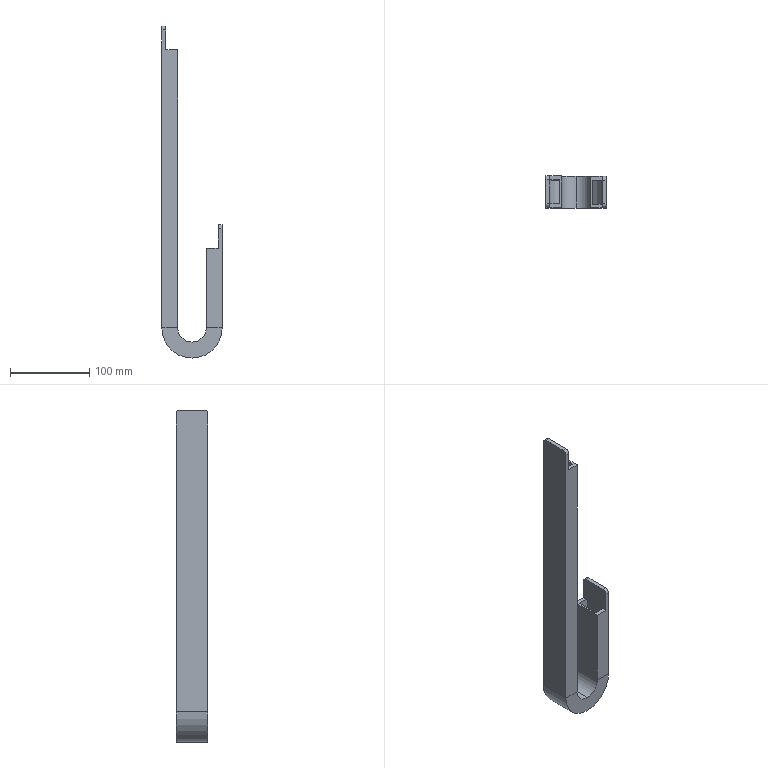Part | SolidWorks | features Fillet 2, ICE 2, Sweep 1, SweepCut 1 | 1 solid | 38 faces | box 76 x 40 x 418 mm | volume 200180 mm3 | plane 28 | cylinder 10 | commonest cylinder face diameters 10 x4 36 x2 76 x2 41 x1 71 x1
STEP:
#1=CARTESIAN_POINT('',(28.,20.,-368.));
#2=VERTEX_POINT('',#1);
#3=CARTESIAN_POINT('',(46.,20.,-350.));
#4=VERTEX_POINT('',#3);
#5=CARTESIAN_POINT('',(28.,20.,-350.));
#6=DIRECTION('',(0.,-1.,0.));
#7=DIRECTION('',(-1.,0.,0.));
#8=AXIS2_PLACEMENT_3D('',#5,#6,#7);
#9=CIRCLE('',#8,18.);
#10=EDGE_CURVE('',#2,#4,#9,.T.);
#11=ORIENTED_EDGE('',*,*,#10,.F.);
#12=CARTESIAN_POINT('',(28.,-20.,-368.));
#13=VERTEX_POINT('',#12);
#14=CARTESIAN_POINT('',(28.,0.,-368.));
#15=DIRECTION('',(0.,-1.,0.));
#16=VECTOR('',#15,1000.);
#17=LINE('',#14,#16);
#18=EDGE_CURVE('',#2,#13,#17,.T.);
#19=ORIENTED_EDGE('',*,*,#18,.T.);
#20=CARTESIAN_POINT('',(46.,-20.,-350.));
#21=VERTEX_POINT('',#20);
#22=CARTESIAN_POINT('',(28.,-20.,-350.));
#23=DIRECTION('',(0.,-1.,0.));
#24=DIRECTION('',(-1.,0.,0.));
#25=AXIS2_PLACEMENT_3D('',#22,#23,#24);
#26=CIRCLE('',#25,18.);
#27=EDGE_CURVE('',#13,#21,#26,.T.);
#28=ORIENTED_EDGE('',*,*,#27,.T.);
#29=CARTESIAN_POINT('',(46.,20.,-350.));
#30=DIRECTION('',(0.,1.,0.));
#31=VECTOR('',#30,1000.);
#32=LINE('',#29,#31);
#33=EDGE_CURVE('',#21,#4,#32,.T.);
#34=ORIENTED_EDGE('',*,*,#33,.T.);
#35=EDGE_LOOP('',(#11,#19,#28,#34));
#36=FACE_OUTER_BOUND('',#35,.T.);
#37=CARTESIAN_POINT('',(28.,0.,-350.));
#38=DIRECTION('',(0.,-1.,0.));
#39=DIRECTION('',(0.,0.,-1.));
#40=AXIS2_PLACEMENT_3D('',#37,#38,#39);
#41=CYLINDRICAL_SURFACE('',#40,18.);
#42=ADVANCED_FACE('',(#36),#41,.F.);
#43=CARTESIAN_POINT('',(-10.,20.,-350.));
#44=VERTEX_POINT('',#43);
#45=CARTESIAN_POINT('',(28.,20.,-388.));
#46=VERTEX_POINT('',#45);
#47=CARTESIAN_POINT('',(28.,20.,-350.));
#48=DIRECTION('',(0.,-1.,0.));
#49=DIRECTION('',(-1.,0.,0.));
#50=AXIS2_PLACEMENT_3D('',#47,#48,#49);
#51=CIRCLE('',#50,38.);
#52=EDGE_CURVE('',#44,#46,#51,.T.);
#53=ORIENTED_EDGE('',*,*,#52,.T.);
#54=CARTESIAN_POINT('',(28.,-20.,-388.));
#55=VERTEX_POINT('',#54);
#56=CARTESIAN_POINT('',(28.,0.,-388.));
#57=DIRECTION('',(0.,-1.,0.));
#58=VECTOR('',#57,1000.);
#59=LINE('',#56,#58);
#60=EDGE_CURVE('',#46,#55,#59,.T.);
#61=ORIENTED_EDGE('',*,*,#60,.T.);
#62=CARTESIAN_POINT('',(-10.,-20.,-350.));
#63=VERTEX_POINT('',#62);
#64=CARTESIAN_POINT('',(28.,-20.,-350.));
#65=DIRECTION('',(0.,-1.,0.));
#66=DIRECTION('',(-1.,0.,0.));
#67=AXIS2_PLACEMENT_3D('',#64,#65,#66);
#68=CIRCLE('',#67,38.);
#69=EDGE_CURVE('',#63,#55,#68,.T.);
#70=ORIENTED_EDGE('',*,*,#69,.F.);
#71=CARTESIAN_POINT('',(-10.,20.,-350.));
#72=DIRECTION('',(0.,-1.,0.));
#73=VECTOR('',#72,1000.);
#74=LINE('',#71,#73);
#75=EDGE_CURVE('',#44,#63,#74,.T.);
#76=ORIENTED_EDGE('',*,*,#75,.F.);
#77=EDGE_LOOP('',(#53,#61,#70,#76));
#78=FACE_OUTER_BOUND('',#77,.T.);
#79=CARTESIAN_POINT('',(28.,0.,-350.));
#80=DIRECTION('',(0.,-1.,0.));
#81=DIRECTION('',(0.,0.,-1.));
#82=AXIS2_PLACEMENT_3D('',#79,#80,#81);
#83=CYLINDRICAL_SURFACE('',#82,38.);
#84=ADVANCED_FACE('',(#78),#83,.T.);
#85=CARTESIAN_POINT('',(61.,20.,-250.));
#86=VERTEX_POINT('',#85);
#87=CARTESIAN_POINT('',(61.,15.,-250.));
#88=VERTEX_POINT('',#87);
#89=CARTESIAN_POINT('',(61.,-20.,-250.));
#90=DIRECTION('',(0.,-1.,0.));
#91=VECTOR('',#90,1000.);
#92=LINE('',#89,#91);
#93=EDGE_CURVE('',#86,#88,#92,.T.);
#94=ORIENTED_EDGE('',*,*,#93,.F.);
#95=CARTESIAN_POINT('',(46.,20.,-250.));
#96=VERTEX_POINT('',#95);
#97=CARTESIAN_POINT('',(66.,20.,-250.));
#98=DIRECTION('',(1.,0.,0.));
#99=VECTOR('',#98,1000.);
#100=LINE('',#97,#99);
#101=EDGE_CURVE('',#96,#86,#100,.T.);
#102=ORIENTED_EDGE('',*,*,#101,.F.);
#103=CARTESIAN_POINT('',(46.,-20.,-250.));
#104=VERTEX_POINT('',#103);
#105=CARTESIAN_POINT('',(46.,20.,-250.));
#106=DIRECTION('',(0.,1.,0.));
#107=VECTOR('',#106,1000.);
#108=LINE('',#105,#107);
#109=EDGE_CURVE('',#104,#96,#108,.T.);
#110=ORIENTED_EDGE('',*,*,#109,.F.);
#111=CARTESIAN_POINT('',(61.,-20.,-250.));
#112=VERTEX_POINT('',#111);
#113=CARTESIAN_POINT('',(66.,-20.,-250.));
#114=DIRECTION('',(-1.,0.,0.));
#115=VECTOR('',#114,1000.);
#116=LINE('',#113,#115);
#117=EDGE_CURVE('',#112,#104,#116,.T.);
#118=ORIENTED_EDGE('',*,*,#117,.F.);
#119=CARTESIAN_POINT('',(61.,-15.,-250.));
#120=VERTEX_POINT('',#119);
#121=CARTESIAN_POINT('',(61.,-20.,-250.));
#122=DIRECTION('',(0.,-1.,0.));
#123=VECTOR('',#122,1000.);
#124=LINE('',#121,#123);
#125=EDGE_CURVE('',#120,#112,#124,.T.);
#126=ORIENTED_EDGE('',*,*,#125,.F.);
#127=CARTESIAN_POINT('',(48.5,-15.,-250.));
#128=VERTEX_POINT('',#127);
#129=CARTESIAN_POINT('',(56.,-15.,-250.));
#130=DIRECTION('',(-1.,0.,0.));
#131=VECTOR('',#130,1000.);
#132=LINE('',#129,#131);
#133=EDGE_CURVE('',#120,#128,#132,.T.);
#134=ORIENTED_EDGE('',*,*,#133,.T.);
#135=CARTESIAN_POINT('',(48.5,15.,-250.));
#136=VERTEX_POINT('',#135);
#137=CARTESIAN_POINT('',(48.5,0.,-250.));
#138=DIRECTION('',(0.,1.,0.));
#139=VECTOR('',#138,1000.);
#140=LINE('',#137,#139);
#141=EDGE_CURVE('',#128,#136,#140,.T.);
#142=ORIENTED_EDGE('',*,*,#141,.T.);
#143=CARTESIAN_POINT('',(56.,15.,-250.));
#144=DIRECTION('',(1.,0.,0.));
#145=VECTOR('',#144,1000.);
#146=LINE('',#143,#145);
#147=EDGE_CURVE('',#136,#88,#146,.T.);
#148=ORIENTED_EDGE('',*,*,#147,.T.);
#149=EDGE_LOOP('',(#94,#102,#110,#118,#126,#134,#142,#148));
#150=FACE_OUTER_BOUND('',#149,.T.);
#151=CARTESIAN_POINT('',(56.,0.,-250.));
#152=DIRECTION('',(0.,0.,-1.));
#153=DIRECTION('',(-1.,0.,0.));
#154=AXIS2_PLACEMENT_3D('',#151,#152,#153);
#155=PLANE('',#154);
#156=ADVANCED_FACE('',(#150),#155,.F.);
#157=CARTESIAN_POINT('',(61.,20.,-225.));
#158=VERTEX_POINT('',#157);
#159=CARTESIAN_POINT('',(61.,20.,-220.));
#160=DIRECTION('',(0.,0.,-1.));
#161=VECTOR('',#160,1000.);
#162=LINE('',#159,#161);
#163=EDGE_CURVE('',#158,#86,#162,.T.);
#164=ORIENTED_EDGE('',*,*,#163,.F.);
#165=CARTESIAN_POINT('',(66.,20.,-225.));
#166=VERTEX_POINT('',#165);
#167=CARTESIAN_POINT('',(66.,20.,-225.));
#168=DIRECTION('',(1.,0.,0.));
#169=VECTOR('',#168,1000.);
#170=LINE('',#167,#169);
#171=EDGE_CURVE('',#158,#166,#170,.T.);
#172=ORIENTED_EDGE('',*,*,#171,.T.);
#173=CARTESIAN_POINT('',(66.,20.,-350.));
#174=VERTEX_POINT('',#173);
#175=CARTESIAN_POINT('',(66.,20.,-350.));
#176=DIRECTION('',(0.,0.,1.));
#177=VECTOR('',#176,1000.);
#178=LINE('',#175,#177);
#179=EDGE_CURVE('',#174,#166,#178,.T.);
#180=ORIENTED_EDGE('',*,*,#179,.F.);
#181=CARTESIAN_POINT('',(66.,20.,-350.));
#182=DIRECTION('',(1.,0.,0.));
#183=VECTOR('',#182,1000.);
#184=LINE('',#181,#183);
#185=EDGE_CURVE('',#4,#174,#184,.T.);
#186=ORIENTED_EDGE('',*,*,#185,.F.);
#187=CARTESIAN_POINT('',(46.,20.,-350.));
#188=DIRECTION('',(0.,0.,1.));
#189=VECTOR('',#188,1000.);
#190=LINE('',#187,#189);
#191=EDGE_CURVE('',#4,#96,#190,.T.);
#192=ORIENTED_EDGE('',*,*,#191,.T.);
#193=ORIENTED_EDGE('',*,*,#101,.T.);
#194=EDGE_LOOP('',(#164,#172,#180,#186,#192,#193));
#195=FACE_OUTER_BOUND('',#194,.T.);
#196=CARTESIAN_POINT('',(66.,20.,-350.));
#197=DIRECTION('',(0.,-1.,0.));
#198=DIRECTION('',(1.,0.,0.));
#199=AXIS2_PLACEMENT_3D('',#196,#197,#198);
#200=PLANE('',#199);
#201=ADVANCED_FACE('',(#195),#200,.F.);
#202=ORIENTED_EDGE('',*,*,#191,.F.);
#203=ORIENTED_EDGE('',*,*,#33,.F.);
#204=CARTESIAN_POINT('',(46.,-20.,-350.));
#205=DIRECTION('',(0.,0.,1.));
#206=VECTOR('',#205,1000.);
#207=LINE('',#204,#206);
#208=EDGE_CURVE('',#21,#104,#207,.T.);
#209=ORIENTED_EDGE('',*,*,#208,.T.);
#210=ORIENTED_EDGE('',*,*,#109,.T.);
#211=EDGE_LOOP('',(#202,#203,#209,#210));
#212=FACE_OUTER_BOUND('',#211,.T.);
#213=CARTESIAN_POINT('',(46.,20.,-350.));
#214=DIRECTION('',(1.,0.,0.));
#215=DIRECTION('',(0.,0.,-1.));
#216=AXIS2_PLACEMENT_3D('',#213,#214,#215);
#217=PLANE('',#216);
#218=ADVANCED_FACE('',(#212),#217,.F.);
#219=CARTESIAN_POINT('',(66.,-20.,-350.));
#220=VERTEX_POINT('',#219);
#221=CARTESIAN_POINT('',(66.,-20.,-225.));
#222=VERTEX_POINT('',#221);
#223=CARTESIAN_POINT('',(66.,-20.,-350.));
#224=DIRECTION('',(0.,0.,1.));
#225=VECTOR('',#224,1000.);
#226=LINE('',#223,#225);
#227=EDGE_CURVE('',#220,#222,#226,.T.);
#228=ORIENTED_EDGE('',*,*,#227,.T.);
#229=CARTESIAN_POINT('',(61.,-20.,-225.));
#230=VERTEX_POINT('',#229);
#231=CARTESIAN_POINT('',(61.,-20.,-225.));
#232=DIRECTION('',(-1.,0.,0.));
#233=VECTOR('',#232,1000.);
#234=LINE('',#231,#233);
#235=EDGE_CURVE('',#222,#230,#234,.T.);
#236=ORIENTED_EDGE('',*,*,#235,.T.);
#237=CARTESIAN_POINT('',(61.,-20.,-220.));
#238=DIRECTION('',(0.,0.,-1.));
#239=VECTOR('',#238,1000.);
#240=LINE('',#237,#239);
#241=EDGE_CURVE('',#230,#112,#240,.T.);
#242=ORIENTED_EDGE('',*,*,#241,.T.);
#243=ORIENTED_EDGE('',*,*,#117,.T.);
#244=ORIENTED_EDGE('',*,*,#208,.F.);
#245=CARTESIAN_POINT('',(66.,-20.,-350.));
#246=DIRECTION('',(-1.,0.,0.));
#247=VECTOR('',#246,1000.);
#248=LINE('',#245,#247);
#249=EDGE_CURVE('',#220,#21,#248,.T.);
#250=ORIENTED_EDGE('',*,*,#249,.F.);
#251=EDGE_LOOP('',(#228,#236,#242,#243,#244,#250));
#252=FACE_OUTER_BOUND('',#251,.T.);
#253=CARTESIAN_POINT('',(66.,-20.,-350.));
#254=DIRECTION('',(0.,1.,0.));
#255=DIRECTION('',(0.,0.,1.));
#256=AXIS2_PLACEMENT_3D('',#253,#254,#255);
#257=PLANE('',#256);
#258=ADVANCED_FACE('',(#252),#257,.F.);
#259=ORIENTED_EDGE('',*,*,#179,.T.);
#260=CARTESIAN_POINT('',(66.,15.,-220.));
#261=VERTEX_POINT('',#260);
#262=CARTESIAN_POINT('',(66.,15.,-225.));
#263=DIRECTION('',(1.,0.,0.));
#264=DIRECTION('',(0.,0.,1.));
#265=AXIS2_PLACEMENT_3D('',#262,#263,#264);
#266=CIRCLE('',#265,5.);
#267=EDGE_CURVE('',#166,#261,#266,.T.);
#268=ORIENTED_EDGE('',*,*,#267,.T.);
#269=CARTESIAN_POINT('',(66.,-15.,-220.));
#270=VERTEX_POINT('',#269);
#271=CARTESIAN_POINT('',(66.,-20.,-220.));
#272=DIRECTION('',(0.,1.,0.));
#273=VECTOR('',#272,1000.);
#274=LINE('',#271,#273);
#275=EDGE_CURVE('',#270,#261,#274,.T.);
#276=ORIENTED_EDGE('',*,*,#275,.F.);
#277=CARTESIAN_POINT('',(66.,-15.,-225.));
#278=DIRECTION('',(1.,0.,0.));
#279=DIRECTION('',(0.,0.,1.));
#280=AXIS2_PLACEMENT_3D('',#277,#278,#279);
#281=CIRCLE('',#280,5.);
#282=EDGE_CURVE('',#270,#222,#281,.T.);
#283=ORIENTED_EDGE('',*,*,#282,.T.);
#284=ORIENTED_EDGE('',*,*,#227,.F.);
#285=CARTESIAN_POINT('',(66.,20.,-350.));
#286=DIRECTION('',(0.,-1.,0.));
#287=VECTOR('',#286,1000.);
#288=LINE('',#285,#287);
#289=EDGE_CURVE('',#174,#220,#288,.T.);
#290=ORIENTED_EDGE('',*,*,#289,.F.);
#291=EDGE_LOOP('',(#259,#268,#276,#283,#284,#290));
#292=FACE_OUTER_BOUND('',#291,.T.);
#293=CARTESIAN_POINT('',(66.,20.,-350.));
#294=DIRECTION('',(-1.,0.,0.));
#295=DIRECTION('',(0.,0.,1.));
#296=AXIS2_PLACEMENT_3D('',#293,#294,#295);
#297=PLANE('',#296);
#298=ADVANCED_FACE('',(#292),#297,.F.);
#299=ORIENTED_EDGE('',*,*,#185,.T.);
#300=CARTESIAN_POINT('',(28.,20.,-350.));
#301=DIRECTION('',(0.,-1.,0.));
#302=DIRECTION('',(-1.,0.,0.));
#303=AXIS2_PLACEMENT_3D('',#300,#301,#302);
#304=CIRCLE('',#303,38.);
#305=EDGE_CURVE('',#46,#174,#304,.T.);
#306=ORIENTED_EDGE('',*,*,#305,.F.);
#307=ORIENTED_EDGE('',*,*,#52,.F.);
#308=CARTESIAN_POINT('',(10.,20.,-350.));
#309=VERTEX_POINT('',#308);
#310=CARTESIAN_POINT('',(-10.,20.,-350.));
#311=DIRECTION('',(-1.,0.,0.));
#312=VECTOR('',#311,1000.);
#313=LINE('',#310,#312);
#314=EDGE_CURVE('',#309,#44,#313,.T.);
#315=ORIENTED_EDGE('',*,*,#314,.F.);
#316=CARTESIAN_POINT('',(28.,20.,-350.));
#317=DIRECTION('',(0.,-1.,0.));
#318=DIRECTION('',(-1.,0.,0.));
#319=AXIS2_PLACEMENT_3D('',#316,#317,#318);
#320=CIRCLE('',#319,18.);
#321=EDGE_CURVE('',#309,#2,#320,.T.);
#322=ORIENTED_EDGE('',*,*,#321,.T.);
#323=ORIENTED_EDGE('',*,*,#10,.T.);
#324=EDGE_LOOP('',(#299,#306,#307,#315,#322,#323));
#325=FACE_OUTER_BOUND('',#324,.T.);
#326=CARTESIAN_POINT('',(-10.,20.,-350.));
#327=DIRECTION('',(0.,-1.,0.));
#328=DIRECTION('',(0.,0.,-1.));
#329=AXIS2_PLACEMENT_3D('',#326,#327,#328);
#330=PLANE('',#329);
#331=ADVANCED_FACE('',(#325),#330,.F.);
#332=ORIENTED_EDGE('',*,*,#18,.F.);
#333=ORIENTED_EDGE('',*,*,#321,.F.);
#334=CARTESIAN_POINT('',(10.,-20.,-350.));
#335=VERTEX_POINT('',#334);
#336=CARTESIAN_POINT('',(10.,20.,-350.));
#337=DIRECTION('',(0.,1.,0.));
#338=VECTOR('',#337,1000.);
#339=LINE('',#336,#338);
#340=EDGE_CURVE('',#335,#309,#339,.T.);
#341=ORIENTED_EDGE('',*,*,#340,.F.);
#342=CARTESIAN_POINT('',(28.,-20.,-350.));
#343=DIRECTION('',(0.,-1.,0.));
#344=DIRECTION('',(-1.,0.,0.));
#345=AXIS2_PLACEMENT_3D('',#342,#343,#344);
#346=CIRCLE('',#345,18.);
#347=EDGE_CURVE('',#335,#13,#346,.T.);
#348=ORIENTED_EDGE('',*,*,#347,.T.);
#349=EDGE_LOOP('',(#332,#333,#341,#348));
#350=FACE_OUTER_BOUND('',#349,.T.);
#351=CARTESIAN_POINT('',(28.,0.,-350.));
#352=DIRECTION('',(0.,-1.,0.));
#353=DIRECTION('',(0.,0.,-1.));
#354=AXIS2_PLACEMENT_3D('',#351,#352,#353);
#355=CYLINDRICAL_SURFACE('',#354,18.);
#356=ADVANCED_FACE('',(#350),#355,.F.);
#357=ORIENTED_EDGE('',*,*,#347,.F.);
#358=CARTESIAN_POINT('',(-10.,-20.,-350.));
#359=DIRECTION('',(1.,0.,0.));
#360=VECTOR('',#359,1000.);
#361=LINE('',#358,#360);
#362=EDGE_CURVE('',#63,#335,#361,.T.);
#363=ORIENTED_EDGE('',*,*,#362,.F.);
#364=ORIENTED_EDGE('',*,*,#69,.T.);
#365=CARTESIAN_POINT('',(28.,-20.,-350.));
#366=DIRECTION('',(0.,-1.,0.));
#367=DIRECTION('',(-1.,0.,0.));
#368=AXIS2_PLACEMENT_3D('',#365,#366,#367);
#369=CIRCLE('',#368,38.);
#370=EDGE_CURVE('',#55,#220,#369,.T.);
#371=ORIENTED_EDGE('',*,*,#370,.T.);
#372=ORIENTED_EDGE('',*,*,#249,.T.);
#373=ORIENTED_EDGE('',*,*,#27,.F.);
#374=EDGE_LOOP('',(#357,#363,#364,#371,#372,#373));
#375=FACE_OUTER_BOUND('',#374,.T.);
#376=CARTESIAN_POINT('',(-10.,-20.,-350.));
#377=DIRECTION('',(0.,1.,0.));
#378=DIRECTION('',(0.,0.,1.));
#379=AXIS2_PLACEMENT_3D('',#376,#377,#378);
#380=PLANE('',#379);
#381=ADVANCED_FACE('',(#375),#380,.F.);
#382=ORIENTED_EDGE('',*,*,#60,.F.);
#383=ORIENTED_EDGE('',*,*,#305,.T.);
#384=ORIENTED_EDGE('',*,*,#289,.T.);
#385=ORIENTED_EDGE('',*,*,#370,.F.);
#386=EDGE_LOOP('',(#382,#383,#384,#385));
#387=FACE_OUTER_BOUND('',#386,.T.);
#388=CARTESIAN_POINT('',(28.,0.,-350.));
#389=DIRECTION('',(0.,-1.,0.));
#390=DIRECTION('',(0.,0.,-1.));
#391=AXIS2_PLACEMENT_3D('',#388,#389,#390);
#392=CYLINDRICAL_SURFACE('',#391,38.);
#393=ADVANCED_FACE('',(#387),#392,.T.);
#394=CARTESIAN_POINT('',(-10.,20.,25.));
#395=VERTEX_POINT('',#394);
#396=CARTESIAN_POINT('',(-10.,20.,0.));
#397=DIRECTION('',(0.,0.,-1.));
#398=VECTOR('',#397,1000.);
#399=LINE('',#396,#398);
#400=EDGE_CURVE('',#395,#44,#399,.T.);
#401=ORIENTED_EDGE('',*,*,#400,.F.);
#402=CARTESIAN_POINT('',(-5.,20.,25.));
#403=VERTEX_POINT('',#402);
#404=CARTESIAN_POINT('',(-10.,20.,25.));
#405=DIRECTION('',(1.,0.,0.));
#406=VECTOR('',#405,1000.);
#407=LINE('',#404,#406);
#408=EDGE_CURVE('',#395,#403,#407,.T.);
#409=ORIENTED_EDGE('',*,*,#408,.T.);
#410=CARTESIAN_POINT('',(-5.,20.,0.));
#411=VERTEX_POINT('',#410);
#412=CARTESIAN_POINT('',(-5.,20.,30.));
#413=DIRECTION('',(0.,0.,-1.));
#414=VECTOR('',#413,1000.);
#415=LINE('',#412,#414);
#416=EDGE_CURVE('',#403,#411,#415,.T.);
#417=ORIENTED_EDGE('',*,*,#416,.T.);
#418=CARTESIAN_POINT('',(10.,20.,0.));
#419=VERTEX_POINT('',#418);
#420=CARTESIAN_POINT('',(-10.,20.,0.));
#421=DIRECTION('',(-1.,0.,0.));
#422=VECTOR('',#421,1000.);
#423=LINE('',#420,#422);
#424=EDGE_CURVE('',#419,#411,#423,.T.);
#425=ORIENTED_EDGE('',*,*,#424,.F.);
#426=CARTESIAN_POINT('',(10.,20.,0.));
#427=DIRECTION('',(0.,0.,-1.));
#428=VECTOR('',#427,1000.);
#429=LINE('',#426,#428);
#430=EDGE_CURVE('',#419,#309,#429,.T.);
#431=ORIENTED_EDGE('',*,*,#430,.T.);
#432=ORIENTED_EDGE('',*,*,#314,.T.);
#433=EDGE_LOOP('',(#401,#409,#417,#425,#431,#432));
#434=FACE_OUTER_BOUND('',#433,.T.);
#435=CARTESIAN_POINT('',(-10.,20.,0.));
#436=DIRECTION('',(0.,-1.,0.));
#437=DIRECTION('',(1.,0.,0.));
#438=AXIS2_PLACEMENT_3D('',#435,#436,#437);
#439=PLANE('',#438);
#440=ADVANCED_FACE('',(#434),#439,.F.);
#441=ORIENTED_EDGE('',*,*,#430,.F.);
#442=CARTESIAN_POINT('',(10.,-20.,0.));
#443=VERTEX_POINT('',#442);
#444=CARTESIAN_POINT('',(10.,20.,0.));
#445=DIRECTION('',(0.,1.,0.));
#446=VECTOR('',#445,1000.);
#447=LINE('',#444,#446);
#448=EDGE_CURVE('',#443,#419,#447,.T.);
#449=ORIENTED_EDGE('',*,*,#448,.F.);
#450=CARTESIAN_POINT('',(10.,-20.,0.));
#451=DIRECTION('',(0.,0.,-1.));
#452=VECTOR('',#451,1000.);
#453=LINE('',#450,#452);
#454=EDGE_CURVE('',#443,#335,#453,.T.);
#455=ORIENTED_EDGE('',*,*,#454,.T.);
#456=ORIENTED_EDGE('',*,*,#340,.T.);
#457=EDGE_LOOP('',(#441,#449,#455,#456));
#458=FACE_OUTER_BOUND('',#457,.T.);
#459=CARTESIAN_POINT('',(10.,20.,0.));
#460=DIRECTION('',(-1.,0.,0.));
#461=DIRECTION('',(0.,-1.,0.));
#462=AXIS2_PLACEMENT_3D('',#459,#460,#461);
#463=PLANE('',#462);
#464=ADVANCED_FACE('',(#458),#463,.F.);
#465=CARTESIAN_POINT('',(-5.,-20.,25.));
#466=VERTEX_POINT('',#465);
#467=CARTESIAN_POINT('',(-5.,-20.,0.));
#468=VERTEX_POINT('',#467);
#469=CARTESIAN_POINT('',(-5.,-20.,30.));
#470=DIRECTION('',(0.,0.,-1.));
#471=VECTOR('',#470,1000.);
#472=LINE('',#469,#471);
#473=EDGE_CURVE('',#466,#468,#472,.T.);
#474=ORIENTED_EDGE('',*,*,#473,.F.);
#475=CARTESIAN_POINT('',(-10.,-20.,25.));
#476=VERTEX_POINT('',#475);
#477=CARTESIAN_POINT('',(-10.,-20.,25.));
#478=DIRECTION('',(-1.,0.,0.));
#479=VECTOR('',#478,1000.);
#480=LINE('',#477,#479);
#481=EDGE_CURVE('',#466,#476,#480,.T.);
#482=ORIENTED_EDGE('',*,*,#481,.T.);
#483=CARTESIAN_POINT('',(-10.,-20.,0.));
#484=DIRECTION('',(0.,0.,-1.));
#485=VECTOR('',#484,1000.);
#486=LINE('',#483,#485);
#487=EDGE_CURVE('',#476,#63,#486,.T.);
#488=ORIENTED_EDGE('',*,*,#487,.T.);
#489=ORIENTED_EDGE('',*,*,#362,.T.);
#490=ORIENTED_EDGE('',*,*,#454,.F.);
#491=CARTESIAN_POINT('',(-10.,-20.,0.));
#492=DIRECTION('',(1.,0.,0.));
#493=VECTOR('',#492,1000.);
#494=LINE('',#491,#493);
#495=EDGE_CURVE('',#468,#443,#494,.T.);
#496=ORIENTED_EDGE('',*,*,#495,.F.);
#497=EDGE_LOOP('',(#474,#482,#488,#489,#490,#496));
#498=FACE_OUTER_BOUND('',#497,.T.);
#499=CARTESIAN_POINT('',(-10.,-20.,0.));
#500=DIRECTION('',(0.,1.,0.));
#501=DIRECTION('',(0.,0.,1.));
#502=AXIS2_PLACEMENT_3D('',#499,#500,#501);
#503=PLANE('',#502);
#504=ADVANCED_FACE('',(#498),#503,.F.);
#505=ORIENTED_EDGE('',*,*,#487,.F.);
#506=CARTESIAN_POINT('',(-10.,-15.,30.));
#507=VERTEX_POINT('',#506);
#508=CARTESIAN_POINT('',(-10.,-15.,25.));
#509=DIRECTION('',(-1.,0.,0.));
#510=DIRECTION('',(0.,1.,0.));
#511=AXIS2_PLACEMENT_3D('',#508,#509,#510);
#512=CIRCLE('',#511,5.);
#513=EDGE_CURVE('',#476,#507,#512,.T.);
#514=ORIENTED_EDGE('',*,*,#513,.T.);
#515=CARTESIAN_POINT('',(-10.,15.,30.));
#516=VERTEX_POINT('',#515);
#517=CARTESIAN_POINT('',(-10.,20.,30.));
#518=DIRECTION('',(0.,-1.,0.));
#519=VECTOR('',#518,1000.);
#520=LINE('',#517,#519);
#521=EDGE_CURVE('',#516,#507,#520,.T.);
#522=ORIENTED_EDGE('',*,*,#521,.F.);
#523=CARTESIAN_POINT('',(-10.,15.,25.));
#524=DIRECTION('',(-1.,0.,0.));
#525=DIRECTION('',(0.,1.,0.));
#526=AXIS2_PLACEMENT_3D('',#523,#524,#525);
#527=CIRCLE('',#526,5.);
#528=EDGE_CURVE('',#516,#395,#527,.T.);
#529=ORIENTED_EDGE('',*,*,#528,.T.);
#530=ORIENTED_EDGE('',*,*,#400,.T.);
#531=ORIENTED_EDGE('',*,*,#75,.T.);
#532=EDGE_LOOP('',(#505,#514,#522,#529,#530,#531));
#533=FACE_OUTER_BOUND('',#532,.T.);
#534=CARTESIAN_POINT('',(-10.,20.,0.));
#535=DIRECTION('',(1.,0.,0.));
#536=DIRECTION('',(0.,1.,0.));
#537=AXIS2_PLACEMENT_3D('',#534,#535,#536);
#538=PLANE('',#537);
#539=ADVANCED_FACE('',(#533),#538,.F.);
#540=CARTESIAN_POINT('',(-5.,-15.,0.));
#541=VERTEX_POINT('',#540);
#542=CARTESIAN_POINT('',(-5.,20.,0.));
#543=DIRECTION('',(0.,1.,0.));
#544=VECTOR('',#543,1000.);
#545=LINE('',#542,#544);
#546=EDGE_CURVE('',#468,#541,#545,.T.);
#547=ORIENTED_EDGE('',*,*,#546,.F.);
#548=ORIENTED_EDGE('',*,*,#495,.T.);
#549=ORIENTED_EDGE('',*,*,#448,.T.);
#550=ORIENTED_EDGE('',*,*,#424,.T.);
#551=CARTESIAN_POINT('',(-5.,15.,0.));
#552=VERTEX_POINT('',#551);
#553=CARTESIAN_POINT('',(-5.,20.,0.));
#554=DIRECTION('',(0.,1.,0.));
#555=VECTOR('',#554,1000.);
#556=LINE('',#553,#555);
#557=EDGE_CURVE('',#552,#411,#556,.T.);
#558=ORIENTED_EDGE('',*,*,#557,.F.);
#559=CARTESIAN_POINT('',(7.5,15.,0.));
#560=VERTEX_POINT('',#559);
#561=CARTESIAN_POINT('',(7.5,15.,0.));
#562=DIRECTION('',(1.,0.,0.));
#563=VECTOR('',#562,1000.);
#564=LINE('',#561,#563);
#565=EDGE_CURVE('',#552,#560,#564,.T.);
#566=ORIENTED_EDGE('',*,*,#565,.T.);
#567=CARTESIAN_POINT('',(7.5,-15.,0.));
#568=VERTEX_POINT('',#567);
#569=CARTESIAN_POINT('',(7.5,15.,0.));
#570=DIRECTION('',(0.,-1.,0.));
#571=VECTOR('',#570,1000.);
#572=LINE('',#569,#571);
#573=EDGE_CURVE('',#560,#568,#572,.T.);
#574=ORIENTED_EDGE('',*,*,#573,.T.);
#575=CARTESIAN_POINT('',(7.5,-15.,0.));
#576=DIRECTION('',(-1.,0.,0.));
#577=VECTOR('',#576,1000.);
#578=LINE('',#575,#577);
#579=EDGE_CURVE('',#568,#541,#578,.T.);
#580=ORIENTED_EDGE('',*,*,#579,.T.);
#581=EDGE_LOOP('',(#547,#548,#549,#550,#558,#566,#574,#580));
#582=FACE_OUTER_BOUND('',#581,.T.);
#583=CARTESIAN_POINT('',(0.,0.,0.));
#584=DIRECTION('',(0.,0.,1.));
#585=DIRECTION('',(1.,0.,0.));
#586=AXIS2_PLACEMENT_3D('',#583,#584,#585);
#587=PLANE('',#586);
#588=ADVANCED_FACE('',(#582),#587,.T.);
#589=CARTESIAN_POINT('',(63.5,15.,-250.));
#590=VERTEX_POINT('',#589);
#591=CARTESIAN_POINT('',(63.5,15.,-350.));
#592=VERTEX_POINT('',#591);
#593=CARTESIAN_POINT('',(63.5,15.,-243.981));
#594=DIRECTION('',(0.,0.,-1.));
#595=VECTOR('',#594,1000.);
#596=LINE('',#593,#595);
#597=EDGE_CURVE('',#590,#592,#596,.T.);
#598=ORIENTED_EDGE('',*,*,#597,.T.);
#599=CARTESIAN_POINT('',(63.5,-15.,-350.));
#600=VERTEX_POINT('',#599);
#601=CARTESIAN_POINT('',(63.5,15.,-350.));
#602=DIRECTION('',(0.,-1.,0.));
#603=VECTOR('',#602,1000.);
#604=LINE('',#601,#603);
#605=EDGE_CURVE('',#592,#600,#604,.T.);
#606=ORIENTED_EDGE('',*,*,#605,.T.);
#607=CARTESIAN_POINT('',(63.5,-15.,-250.));
#608=VERTEX_POINT('',#607);
#609=CARTESIAN_POINT('',(63.5,-15.,-243.981));
#610=DIRECTION('',(0.,0.,-1.));
#611=VECTOR('',#610,1000.);
#612=LINE('',#609,#611);
#613=EDGE_CURVE('',#608,#600,#612,.T.);
#614=ORIENTED_EDGE('',*,*,#613,.F.);
#615=CARTESIAN_POINT('',(63.5,0.,-250.));
#616=DIRECTION('',(0.,-1.,0.));
#617=VECTOR('',#616,1000.);
#618=LINE('',#615,#617);
#619=EDGE_CURVE('',#590,#608,#618,.T.);
#620=ORIENTED_EDGE('',*,*,#619,.F.);
#621=EDGE_LOOP('',(#598,#606,#614,#620));
#622=FACE_OUTER_BOUND('',#621,.T.);
#623=CARTESIAN_POINT('',(63.5,15.,-243.981));
#624=DIRECTION('',(1.,0.,0.));
#625=DIRECTION('',(0.,1.,0.));
#626=AXIS2_PLACEMENT_3D('',#623,#624,#625);
#627=PLANE('',#626);
#628=ADVANCED_FACE('',(#622),#627,.F.);
#629=ORIENTED_EDGE('',*,*,#613,.T.);
#630=CARTESIAN_POINT('',(48.5,-15.,-350.));
#631=VERTEX_POINT('',#630);
#632=CARTESIAN_POINT('',(48.5,-15.,-350.));
#633=DIRECTION('',(-1.,0.,0.));
#634=VECTOR('',#633,1000.);
#635=LINE('',#632,#634);
#636=EDGE_CURVE('',#600,#631,#635,.T.);
#637=ORIENTED_EDGE('',*,*,#636,.T.);
#638=CARTESIAN_POINT('',(48.5,-15.,-243.981));
#639=DIRECTION('',(0.,0.,-1.));
#640=VECTOR('',#639,1000.);
#641=LINE('',#638,#640);
#642=EDGE_CURVE('',#128,#631,#641,.T.);
#643=ORIENTED_EDGE('',*,*,#642,.F.);
#644=ORIENTED_EDGE('',*,*,#133,.F.);
#645=CARTESIAN_POINT('',(56.,-15.,-250.));
#646=DIRECTION('',(-1.,0.,0.));
#647=VECTOR('',#646,1000.);
#648=LINE('',#645,#647);
#649=EDGE_CURVE('',#608,#120,#648,.T.);
#650=ORIENTED_EDGE('',*,*,#649,.F.);
#651=EDGE_LOOP('',(#629,#637,#643,#644,#650));
#652=FACE_OUTER_BOUND('',#651,.T.);
#653=CARTESIAN_POINT('',(48.5,-15.,-243.981));
#654=DIRECTION('',(0.,-1.,0.));
#655=DIRECTION('',(0.,0.,-1.));
#656=AXIS2_PLACEMENT_3D('',#653,#654,#655);
#657=PLANE('',#656);
#658=ADVANCED_FACE('',(#652),#657,.F.);
#659=ORIENTED_EDGE('',*,*,#642,.T.);
#660=CARTESIAN_POINT('',(48.5,15.,-350.));
#661=VERTEX_POINT('',#660);
#662=CARTESIAN_POINT('',(48.5,15.,-350.));
#663=DIRECTION('',(0.,1.,0.));
#664=VECTOR('',#663,1000.);
#665=LINE('',#662,#664);
#666=EDGE_CURVE('',#631,#661,#665,.T.);
#667=ORIENTED_EDGE('',*,*,#666,.T.);
#668=CARTESIAN_POINT('',(48.5,15.,-243.981));
#669=DIRECTION('',(0.,0.,-1.));
#670=VECTOR('',#669,1000.);
#671=LINE('',#668,#670);
#672=EDGE_CURVE('',#136,#661,#671,.T.);
#673=ORIENTED_EDGE('',*,*,#672,.F.);
#674=ORIENTED_EDGE('',*,*,#141,.F.);
#675=EDGE_LOOP('',(#659,#667,#673,#674));
#676=FACE_OUTER_BOUND('',#675,.T.);
#677=CARTESIAN_POINT('',(48.5,15.,-243.981));
#678=DIRECTION('',(-1.,0.,0.));
#679=DIRECTION('',(0.,-1.,0.));
#680=AXIS2_PLACEMENT_3D('',#677,#678,#679);
#681=PLANE('',#680);
#682=ADVANCED_FACE('',(#676),#681,.F.);
#683=ORIENTED_EDGE('',*,*,#672,.T.);
#684=CARTESIAN_POINT('',(48.5,15.,-350.));
#685=DIRECTION('',(1.,0.,0.));
#686=VECTOR('',#685,1000.);
#687=LINE('',#684,#686);
#688=EDGE_CURVE('',#661,#592,#687,.T.);
#689=ORIENTED_EDGE('',*,*,#688,.T.);
#690=ORIENTED_EDGE('',*,*,#597,.F.);
#691=CARTESIAN_POINT('',(56.,15.,-250.));
#692=DIRECTION('',(1.,0.,0.));
#693=VECTOR('',#692,1000.);
#694=LINE('',#691,#693);
#695=EDGE_CURVE('',#88,#590,#694,.T.);
#696=ORIENTED_EDGE('',*,*,#695,.F.);
#697=ORIENTED_EDGE('',*,*,#147,.F.);
#698=EDGE_LOOP('',(#683,#689,#690,#696,#697));
#699=FACE_OUTER_BOUND('',#698,.T.);
#700=CARTESIAN_POINT('',(48.5,15.,-243.981));
#701=DIRECTION('',(0.,1.,0.));
#702=DIRECTION('',(0.,0.,1.));
#703=AXIS2_PLACEMENT_3D('',#700,#701,#702);
#704=PLANE('',#703);
#705=ADVANCED_FACE('',(#699),#704,.F.);
#706=CARTESIAN_POINT('',(-7.5,-15.,-350.));
#707=VERTEX_POINT('',#706);
#708=CARTESIAN_POINT('',(-7.5,-15.,0.));
#709=VERTEX_POINT('',#708);
#710=CARTESIAN_POINT('',(-7.5,-15.,-350.));
#711=DIRECTION('',(0.,0.,1.));
#712=VECTOR('',#711,1000.);
#713=LINE('',#710,#712);
#714=EDGE_CURVE('',#707,#709,#713,.T.);
#715=ORIENTED_EDGE('',*,*,#714,.F.);
#716=CARTESIAN_POINT('',(-7.5,15.,-350.));
#717=VERTEX_POINT('',#716);
#718=CARTESIAN_POINT('',(-7.5,15.,-350.));
#719=DIRECTION('',(0.,-1.,0.));
#720=VECTOR('',#719,1000.);
#721=LINE('',#718,#720);
#722=EDGE_CURVE('',#717,#707,#721,.T.);
#723=ORIENTED_EDGE('',*,*,#722,.F.);
#724=CARTESIAN_POINT('',(-7.5,15.,0.));
#725=VERTEX_POINT('',#724);
#726=CARTESIAN_POINT('',(-7.5,15.,-350.));
#727=DIRECTION('',(0.,0.,1.));
#728=VECTOR('',#727,1000.);
#729=LINE('',#726,#728);
#730=EDGE_CURVE('',#717,#725,#729,.T.);
#731=ORIENTED_EDGE('',*,*,#730,.T.);
#732=CARTESIAN_POINT('',(-7.5,15.,0.));
#733=DIRECTION('',(0.,1.,0.));
#734=VECTOR('',#733,1000.);
#735=LINE('',#732,#734);
#736=EDGE_CURVE('',#709,#725,#735,.T.);
#737=ORIENTED_EDGE('',*,*,#736,.F.);
#738=EDGE_LOOP('',(#715,#723,#731,#737));
#739=FACE_OUTER_BOUND('',#738,.T.);
#740=CARTESIAN_POINT('',(-7.5,15.,-350.));
#741=DIRECTION('',(-1.,0.,0.));
#742=DIRECTION('',(0.,-1.,0.));
#743=AXIS2_PLACEMENT_3D('',#740,#741,#742);
#744=PLANE('',#743);
#745=ADVANCED_FACE('',(#739),#744,.F.);
#746=CARTESIAN_POINT('',(7.5,-15.,-350.));
#747=VERTEX_POINT('',#746);
#748=CARTESIAN_POINT('',(7.5,-15.,-350.));
#749=DIRECTION('',(0.,0.,1.));
#750=VECTOR('',#749,1000.);
#751=LINE('',#748,#750);
#752=EDGE_CURVE('',#747,#568,#751,.T.);
#753=ORIENTED_EDGE('',*,*,#752,.F.);
#754=CARTESIAN_POINT('',(7.5,-15.,-350.));
#755=DIRECTION('',(1.,0.,0.));
#756=VECTOR('',#755,1000.);
#757=LINE('',#754,#756);
#758=EDGE_CURVE('',#707,#747,#757,.T.);
#759=ORIENTED_EDGE('',*,*,#758,.F.);
#760=ORIENTED_EDGE('',*,*,#714,.T.);
#761=CARTESIAN_POINT('',(7.5,-15.,0.));
#762=DIRECTION('',(-1.,0.,0.));
#763=VECTOR('',#762,1000.);
#764=LINE('',#761,#763);
#765=EDGE_CURVE('',#541,#709,#764,.T.);
#766=ORIENTED_EDGE('',*,*,#765,.F.);
#767=ORIENTED_EDGE('',*,*,#579,.F.);
#768=EDGE_LOOP('',(#753,#759,#760,#766,#767));
#769=FACE_OUTER_BOUND('',#768,.T.);
#770=CARTESIAN_POINT('',(7.5,-15.,-350.));
#771=DIRECTION('',(0.,-1.,0.));
#772=DIRECTION('',(0.,0.,-1.));
#773=AXIS2_PLACEMENT_3D('',#770,#771,#772);
#774=PLANE('',#773);
#775=ADVANCED_FACE('',(#769),#774,.F.);
#776=CARTESIAN_POINT('',(7.5,15.,-350.));
#777=VERTEX_POINT('',#776);
#778=CARTESIAN_POINT('',(7.5,15.,-350.));
#779=DIRECTION('',(0.,0.,1.));
#780=VECTOR('',#779,1000.);
#781=LINE('',#778,#780);
#782=EDGE_CURVE('',#777,#560,#781,.T.);
#783=ORIENTED_EDGE('',*,*,#782,.F.);
#784=CARTESIAN_POINT('',(7.5,15.,-350.));
#785=DIRECTION('',(0.,1.,0.));
#786=VECTOR('',#785,1000.);
#787=LINE('',#784,#786);
#788=EDGE_CURVE('',#747,#777,#787,.T.);
#789=ORIENTED_EDGE('',*,*,#788,.F.);
#790=ORIENTED_EDGE('',*,*,#752,.T.);
#791=ORIENTED_EDGE('',*,*,#573,.F.);
#792=EDGE_LOOP('',(#783,#789,#790,#791));
#793=FACE_OUTER_BOUND('',#792,.T.);
#794=CARTESIAN_POINT('',(7.5,15.,-350.));
#795=DIRECTION('',(1.,0.,0.));
#796=DIRECTION('',(0.,1.,0.));
#797=AXIS2_PLACEMENT_3D('',#794,#795,#796);
#798=PLANE('',#797);
#799=ADVANCED_FACE('',(#793),#798,.F.);
#800=ORIENTED_EDGE('',*,*,#730,.F.);
#801=CARTESIAN_POINT('',(7.5,15.,-350.));
#802=DIRECTION('',(-1.,0.,0.));
#803=VECTOR('',#802,1000.);
#804=LINE('',#801,#803);
#805=EDGE_CURVE('',#777,#717,#804,.T.);
#806=ORIENTED_EDGE('',*,*,#805,.F.);
#807=ORIENTED_EDGE('',*,*,#782,.T.);
#808=ORIENTED_EDGE('',*,*,#565,.F.);
#809=CARTESIAN_POINT('',(7.5,15.,0.));
#810=DIRECTION('',(1.,0.,0.));
#811=VECTOR('',#810,1000.);
#812=LINE('',#809,#811);
#813=EDGE_CURVE('',#725,#552,#812,.T.);
#814=ORIENTED_EDGE('',*,*,#813,.F.);
#815=EDGE_LOOP('',(#800,#806,#807,#808,#814));
#816=FACE_OUTER_BOUND('',#815,.T.);
#817=CARTESIAN_POINT('',(7.5,15.,-350.));
#818=DIRECTION('',(0.,1.,0.));
#819=DIRECTION('',(0.,0.,1.));
#820=AXIS2_PLACEMENT_3D('',#817,#818,#819);
#821=PLANE('',#820);
#822=ADVANCED_FACE('',(#816),#821,.F.);
#823=ORIENTED_EDGE('',*,*,#805,.T.);
#824=CARTESIAN_POINT('',(28.,15.,-350.));
#825=DIRECTION('',(0.,1.,0.));
#826=DIRECTION('',(1.,0.,0.));
#827=AXIS2_PLACEMENT_3D('',#824,#825,#826);
#828=CIRCLE('',#827,35.5);
#829=EDGE_CURVE('',#592,#717,#828,.T.);
#830=ORIENTED_EDGE('',*,*,#829,.F.);
#831=ORIENTED_EDGE('',*,*,#688,.F.);
#832=CARTESIAN_POINT('',(28.,15.,-350.));
#833=DIRECTION('',(0.,1.,0.));
#834=DIRECTION('',(1.,0.,0.));
#835=AXIS2_PLACEMENT_3D('',#832,#833,#834);
#836=CIRCLE('',#835,20.5);
#837=EDGE_CURVE('',#661,#777,#836,.T.);
#838=ORIENTED_EDGE('',*,*,#837,.T.);
#839=EDGE_LOOP('',(#823,#830,#831,#838));
#840=FACE_OUTER_BOUND('',#839,.T.);
#841=CARTESIAN_POINT('',(48.5,15.,-350.));
#842=DIRECTION('',(0.,1.,0.));
#843=DIRECTION('',(0.,0.,1.));
#844=AXIS2_PLACEMENT_3D('',#841,#842,#843);
#845=PLANE('',#844);
#846=ADVANCED_FACE('',(#840),#845,.F.);
#847=ORIENTED_EDGE('',*,*,#837,.F.);
#848=ORIENTED_EDGE('',*,*,#666,.F.);
#849=CARTESIAN_POINT('',(28.,-15.,-350.));
#850=DIRECTION('',(0.,1.,0.));
#851=DIRECTION('',(1.,0.,0.));
#852=AXIS2_PLACEMENT_3D('',#849,#850,#851);
#853=CIRCLE('',#852,20.5);
#854=EDGE_CURVE('',#631,#747,#853,.T.);
#855=ORIENTED_EDGE('',*,*,#854,.T.);
#856=ORIENTED_EDGE('',*,*,#788,.T.);
#857=EDGE_LOOP('',(#847,#848,#855,#856));
#858=FACE_OUTER_BOUND('',#857,.T.);
#859=CARTESIAN_POINT('',(28.,0.,-350.));
#860=DIRECTION('',(0.,1.,0.));
#861=DIRECTION('',(0.,0.,1.));
#862=AXIS2_PLACEMENT_3D('',#859,#860,#861);
#863=CYLINDRICAL_SURFACE('',#862,20.5);
#864=ADVANCED_FACE('',(#858),#863,.T.);
#865=ORIENTED_EDGE('',*,*,#854,.F.);
#866=ORIENTED_EDGE('',*,*,#636,.F.);
#867=CARTESIAN_POINT('',(28.,-15.,-350.));
#868=DIRECTION('',(0.,1.,0.));
#869=DIRECTION('',(1.,0.,0.));
#870=AXIS2_PLACEMENT_3D('',#867,#868,#869);
#871=CIRCLE('',#870,35.5);
#872=EDGE_CURVE('',#600,#707,#871,.T.);
#873=ORIENTED_EDGE('',*,*,#872,.T.);
#874=ORIENTED_EDGE('',*,*,#758,.T.);
#875=EDGE_LOOP('',(#865,#866,#873,#874));
#876=FACE_OUTER_BOUND('',#875,.T.);
#877=CARTESIAN_POINT('',(48.5,-15.,-350.));
#878=DIRECTION('',(0.,-1.,0.));
#879=DIRECTION('',(0.,0.,-1.));
#880=AXIS2_PLACEMENT_3D('',#877,#878,#879);
#881=PLANE('',#880);
#882=ADVANCED_FACE('',(#876),#881,.F.);
#883=ORIENTED_EDGE('',*,*,#872,.F.);
#884=ORIENTED_EDGE('',*,*,#605,.F.);
#885=ORIENTED_EDGE('',*,*,#829,.T.);
#886=ORIENTED_EDGE('',*,*,#722,.T.);
#887=EDGE_LOOP('',(#883,#884,#885,#886));
#888=FACE_OUTER_BOUND('',#887,.T.);
#889=CARTESIAN_POINT('',(28.,0.,-350.));
#890=DIRECTION('',(0.,1.,0.));
#891=DIRECTION('',(0.,0.,1.));
#892=AXIS2_PLACEMENT_3D('',#889,#890,#891);
#893=CYLINDRICAL_SURFACE('',#892,35.5);
#894=ADVANCED_FACE('',(#888),#893,.F.);
#895=CARTESIAN_POINT('',(-5.,-15.,30.));
#896=VERTEX_POINT('',#895);
#897=CARTESIAN_POINT('',(-5.,15.,30.));
#898=VERTEX_POINT('',#897);
#899=CARTESIAN_POINT('',(-5.,20.,30.));
#900=DIRECTION('',(0.,1.,0.));
#901=VECTOR('',#900,1000.);
#902=LINE('',#899,#901);
#903=EDGE_CURVE('',#896,#898,#902,.T.);
#904=ORIENTED_EDGE('',*,*,#903,.F.);
#905=CARTESIAN_POINT('',(-5.,-15.,25.));
#906=DIRECTION('',(1.,0.,0.));
#907=DIRECTION('',(0.,-1.,0.));
#908=AXIS2_PLACEMENT_3D('',#905,#906,#907);
#909=CIRCLE('',#908,5.);
#910=EDGE_CURVE('',#896,#466,#909,.T.);
#911=ORIENTED_EDGE('',*,*,#910,.T.);
#912=ORIENTED_EDGE('',*,*,#473,.T.);
#913=ORIENTED_EDGE('',*,*,#546,.T.);
#914=CARTESIAN_POINT('',(-5.,20.,0.));
#915=DIRECTION('',(0.,1.,0.));
#916=VECTOR('',#915,1000.);
#917=LINE('',#914,#916);
#918=EDGE_CURVE('',#541,#552,#917,.T.);
#919=ORIENTED_EDGE('',*,*,#918,.T.);
#920=ORIENTED_EDGE('',*,*,#557,.T.);
#921=ORIENTED_EDGE('',*,*,#416,.F.);
#922=CARTESIAN_POINT('',(-5.,15.,25.));
#923=DIRECTION('',(1.,0.,0.));
#924=DIRECTION('',(0.,-1.,0.));
#925=AXIS2_PLACEMENT_3D('',#922,#923,#924);
#926=CIRCLE('',#925,5.);
#927=EDGE_CURVE('',#403,#898,#926,.T.);
#928=ORIENTED_EDGE('',*,*,#927,.T.);
#929=EDGE_LOOP('',(#904,#911,#912,#913,#919,#920,#921,#928));
#930=FACE_OUTER_BOUND('',#929,.T.);
#931=CARTESIAN_POINT('',(-5.,20.,30.));
#932=DIRECTION('',(-1.,0.,0.));
#933=DIRECTION('',(0.,-1.,0.));
#934=AXIS2_PLACEMENT_3D('',#931,#932,#933);
#935=PLANE('',#934);
#936=ADVANCED_FACE('',(#930),#935,.F.);
#937=ORIENTED_EDGE('',*,*,#521,.T.);
#938=CARTESIAN_POINT('',(0.,-15.,30.));
#939=DIRECTION('',(1.,0.,0.));
#940=VECTOR('',#939,1000.);
#941=LINE('',#938,#940);
#942=EDGE_CURVE('',#507,#896,#941,.T.);
#943=ORIENTED_EDGE('',*,*,#942,.T.);
#944=ORIENTED_EDGE('',*,*,#903,.T.);
#945=CARTESIAN_POINT('',(0.,15.,30.));
#946=DIRECTION('',(-1.,0.,0.));
#947=VECTOR('',#946,1000.);
#948=LINE('',#945,#947);
#949=EDGE_CURVE('',#898,#516,#948,.T.);
#950=ORIENTED_EDGE('',*,*,#949,.T.);
#951=EDGE_LOOP('',(#937,#943,#944,#950));
#952=FACE_OUTER_BOUND('',#951,.T.);
#953=CARTESIAN_POINT('',(0.,0.,30.));
#954=DIRECTION('',(0.,0.,-1.));
#955=DIRECTION('',(-1.,0.,0.));
#956=AXIS2_PLACEMENT_3D('',#953,#954,#955);
#957=PLANE('',#956);
#958=ADVANCED_FACE('',(#952),#957,.F.);
#959=ORIENTED_EDGE('',*,*,#736,.T.);
#960=ORIENTED_EDGE('',*,*,#813,.T.);
#961=ORIENTED_EDGE('',*,*,#918,.F.);
#962=ORIENTED_EDGE('',*,*,#765,.T.);
#963=EDGE_LOOP('',(#959,#960,#961,#962));
#964=FACE_OUTER_BOUND('',#963,.T.);
#965=CARTESIAN_POINT('',(0.,0.,0.));
#966=DIRECTION('',(0.,0.,-1.));
#967=DIRECTION('',(-1.,0.,0.));
#968=AXIS2_PLACEMENT_3D('',#965,#966,#967);
#969=PLANE('',#968);
#970=ADVANCED_FACE('',(#964),#969,.T.);
#971=ORIENTED_EDGE('',*,*,#513,.F.);
#972=ORIENTED_EDGE('',*,*,#481,.F.);
#973=ORIENTED_EDGE('',*,*,#910,.F.);
#974=ORIENTED_EDGE('',*,*,#942,.F.);
#975=EDGE_LOOP('',(#971,#972,#973,#974));
#976=FACE_OUTER_BOUND('',#975,.T.);
#977=CARTESIAN_POINT('',(0.,-15.,25.));
#978=DIRECTION('',(1.,0.,0.));
#979=DIRECTION('',(0.,0.,-1.));
#980=AXIS2_PLACEMENT_3D('',#977,#978,#979);
#981=CYLINDRICAL_SURFACE('',#980,5.);
#982=ADVANCED_FACE('',(#976),#981,.T.);
#983=ORIENTED_EDGE('',*,*,#927,.F.);
#984=ORIENTED_EDGE('',*,*,#408,.F.);
#985=ORIENTED_EDGE('',*,*,#528,.F.);
#986=ORIENTED_EDGE('',*,*,#949,.F.);
#987=EDGE_LOOP('',(#983,#984,#985,#986));
#988=FACE_OUTER_BOUND('',#987,.T.);
#989=CARTESIAN_POINT('',(0.,15.,25.));
#990=DIRECTION('',(-1.,0.,0.));
#991=DIRECTION('',(0.,-1.,0.));
#992=AXIS2_PLACEMENT_3D('',#989,#990,#991);
#993=CYLINDRICAL_SURFACE('',#992,5.);
#994=ADVANCED_FACE('',(#988),#993,.T.);
#995=CARTESIAN_POINT('',(61.,-20.,-250.));
#996=DIRECTION('',(0.,-1.,0.));
#997=VECTOR('',#996,1000.);
#998=LINE('',#995,#997);
#999=EDGE_CURVE('',#88,#120,#998,.T.);
#1000=ORIENTED_EDGE('',*,*,#999,.F.);
#1001=ORIENTED_EDGE('',*,*,#695,.T.);
#1002=ORIENTED_EDGE('',*,*,#619,.T.);
#1003=ORIENTED_EDGE('',*,*,#649,.T.);
#1004=EDGE_LOOP('',(#1000,#1001,#1002,#1003));
#1005=FACE_OUTER_BOUND('',#1004,.T.);
#1006=CARTESIAN_POINT('',(0.,0.,-250.));
#1007=DIRECTION('',(0.,0.,1.));
#1008=DIRECTION('',(1.,0.,0.));
#1009=AXIS2_PLACEMENT_3D('',#1006,#1007,#1008);
#1010=PLANE('',#1009);
#1011=ADVANCED_FACE('',(#1005),#1010,.F.);
#1012=CARTESIAN_POINT('',(61.,15.,-220.));
#1013=VERTEX_POINT('',#1012);
#1014=CARTESIAN_POINT('',(61.,-15.,-220.));
#1015=VERTEX_POINT('',#1014);
#1016=CARTESIAN_POINT('',(61.,-20.,-220.));
#1017=DIRECTION('',(0.,-1.,0.));
#1018=VECTOR('',#1017,1000.);
#1019=LINE('',#1016,#1018);
#1020=EDGE_CURVE('',#1013,#1015,#1019,.T.);
#1021=ORIENTED_EDGE('',*,*,#1020,.F.);
#1022=CARTESIAN_POINT('',(61.,15.,-225.));
#1023=DIRECTION('',(-1.,0.,0.));
#1024=DIRECTION('',(0.,0.,-1.));
#1025=AXIS2_PLACEMENT_3D('',#1022,#1023,#1024);
#1026=CIRCLE('',#1025,5.);
#1027=EDGE_CURVE('',#1013,#158,#1026,.T.);
#1028=ORIENTED_EDGE('',*,*,#1027,.T.);
#1029=ORIENTED_EDGE('',*,*,#163,.T.);
#1030=ORIENTED_EDGE('',*,*,#93,.T.);
#1031=ORIENTED_EDGE('',*,*,#999,.T.);
#1032=ORIENTED_EDGE('',*,*,#125,.T.);
#1033=ORIENTED_EDGE('',*,*,#241,.F.);
#1034=CARTESIAN_POINT('',(61.,-15.,-225.));
#1035=DIRECTION('',(-1.,0.,0.));
#1036=DIRECTION('',(0.,0.,-1.));
#1037=AXIS2_PLACEMENT_3D('',#1034,#1035,#1036);
#1038=CIRCLE('',#1037,5.);
#1039=EDGE_CURVE('',#230,#1015,#1038,.T.);
#1040=ORIENTED_EDGE('',*,*,#1039,.T.);
#1041=EDGE_LOOP('',(#1021,#1028,#1029,#1030,#1031,#1032,#1033,#1040));
#1042=FACE_OUTER_BOUND('',#1041,.T.);
#1043=CARTESIAN_POINT('',(61.,-20.,-220.));
#1044=DIRECTION('',(1.,0.,0.));
#1045=DIRECTION('',(0.,0.,-1.));
#1046=AXIS2_PLACEMENT_3D('',#1043,#1044,#1045);
#1047=PLANE('',#1046);
#1048=ADVANCED_FACE('',(#1042),#1047,.F.);
#1049=ORIENTED_EDGE('',*,*,#275,.T.);
#1050=CARTESIAN_POINT('',(61.,15.,-220.));
#1051=DIRECTION('',(-1.,0.,0.));
#1052=VECTOR('',#1051,1000.);
#1053=LINE('',#1050,#1052);
#1054=EDGE_CURVE('',#261,#1013,#1053,.T.);
#1055=ORIENTED_EDGE('',*,*,#1054,.T.);
#1056=ORIENTED_EDGE('',*,*,#1020,.T.);
#1057=CARTESIAN_POINT('',(66.,-15.,-220.));
#1058=DIRECTION('',(1.,0.,0.));
#1059=VECTOR('',#1058,1000.);
#1060=LINE('',#1057,#1059);
#1061=EDGE_CURVE('',#1015,#270,#1060,.T.);
#1062=ORIENTED_EDGE('',*,*,#1061,.T.);
#1063=EDGE_LOOP('',(#1049,#1055,#1056,#1062));
#1064=FACE_OUTER_BOUND('',#1063,.T.);
#1065=CARTESIAN_POINT('',(0.,0.,-220.));
#1066=DIRECTION('',(0.,0.,1.));
#1067=DIRECTION('',(1.,0.,0.));
#1068=AXIS2_PLACEMENT_3D('',#1065,#1066,#1067);
#1069=PLANE('',#1068);
#1070=ADVANCED_FACE('',(#1064),#1069,.T.);
#1071=ORIENTED_EDGE('',*,*,#267,.F.);
#1072=ORIENTED_EDGE('',*,*,#171,.F.);
#1073=ORIENTED_EDGE('',*,*,#1027,.F.);
#1074=ORIENTED_EDGE('',*,*,#1054,.F.);
#1075=EDGE_LOOP('',(#1071,#1072,#1073,#1074));
#1076=FACE_OUTER_BOUND('',#1075,.T.);
#1077=CARTESIAN_POINT('',(0.,15.,-225.));
#1078=DIRECTION('',(1.,0.,0.));
#1079=DIRECTION('',(0.,1.,0.));
#1080=AXIS2_PLACEMENT_3D('',#1077,#1078,#1079);
#1081=CYLINDRICAL_SURFACE('',#1080,5.);
#1082=ADVANCED_FACE('',(#1076),#1081,.T.);
#1083=ORIENTED_EDGE('',*,*,#1039,.F.);
#1084=ORIENTED_EDGE('',*,*,#235,.F.);
#1085=ORIENTED_EDGE('',*,*,#282,.F.);
#1086=ORIENTED_EDGE('',*,*,#1061,.F.);
#1087=EDGE_LOOP('',(#1083,#1084,#1085,#1086));
#1088=FACE_OUTER_BOUND('',#1087,.T.);
#1089=CARTESIAN_POINT('',(0.,-15.,-225.));
#1090=DIRECTION('',(-1.,0.,0.));
#1091=DIRECTION('',(0.,0.,1.));
#1092=AXIS2_PLACEMENT_3D('',#1089,#1090,#1091);
#1093=CYLINDRICAL_SURFACE('',#1092,5.);
#1094=ADVANCED_FACE('',(#1088),#1093,.T.);
#1095=CLOSED_SHELL('',(#42,#84,#156,#201,#218,#258,#298,#331,#356,#381,#393,#440,#464,#504,#539,#588,#628,#658,#682,#705,#745,#775,#799,#822,#846,#864,#882,#894,#936,#958,#970,#982,#994,#1011,#1048,#1070,#1082,#1094));
#1096=MANIFOLD_SOLID_BREP('',#1095);
#1097=CARTESIAN_POINT('',(0.,0.,0.));
#1098=DIRECTION('',(0.,0.,1.));
#1099=DIRECTION('',(1.,0.,0.));
#1100=AXIS2_PLACEMENT_3D('',#1097,#1098,#1099);
#1101=(LENGTH_UNIT()NAMED_UNIT(*)SI_UNIT(.MILLI.,.METRE.));
#1102=UNCERTAINTY_MEASURE_WITH_UNIT(LENGTH_MEASURE(0.00001),#1101,'','');
#1103=(NAMED_UNIT(*)PLANE_ANGLE_UNIT()SI_UNIT($,.RADIAN.));
#1104=(NAMED_UNIT(*)SI_UNIT($,.STERADIAN.)SOLID_ANGLE_UNIT());
#1105=(GEOMETRIC_REPRESENTATION_CONTEXT(3)GLOBAL_UNCERTAINTY_ASSIGNED_CONTEXT((#1102))GLOBAL_UNIT_ASSIGNED_CONTEXT((#1101,#1103,#1104))REPRESENTATION_CONTEXT('',''));
#1106=ADVANCED_BREP_SHAPE_REPRESENTATION('',(#1096,#1100),#1105);